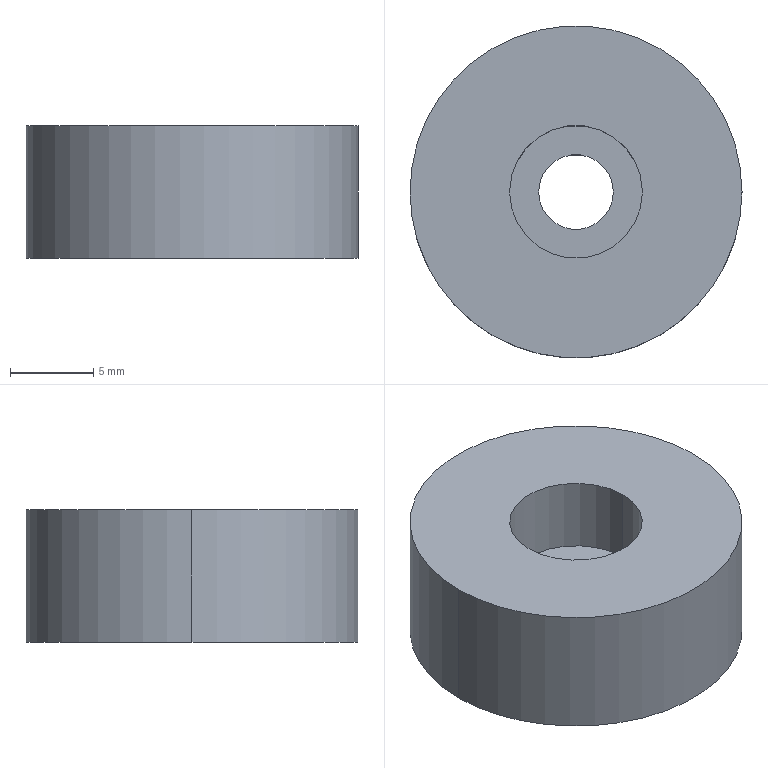Part | STEP file | X77-04005 | 1 solid | 12 faces | box 20 x 20 x 8 mm | volume 2090 mm3 | cylinder 8 | plane 4 | commonest cylinder face diameters 4.5 x2 8 x2 14 x2 20 x2
STEP:
#1=CARTESIAN_POINT('',(7.,0.,1.));
#2=VERTEX_POINT('',#1);
#3=CARTESIAN_POINT('',(-7.,0.,1.));
#4=VERTEX_POINT('',#3);
#5=CARTESIAN_POINT('',(0.,0.,1.));
#6=DIRECTION('',(0.,0.,-1.));
#7=DIRECTION('',(-1.,0.,0.));
#8=AXIS2_PLACEMENT_3D('',#5,#6,#7);
#9=CIRCLE('',#8,7.);
#10=EDGE_CURVE('',#2,#4,#9,.T.);
#11=ORIENTED_EDGE('',*,*,#10,.F.);
#12=CARTESIAN_POINT('',(7.,0.,0.));
#13=VERTEX_POINT('',#12);
#14=CARTESIAN_POINT('',(7.,0.,1.));
#15=DIRECTION('',(0.,0.,-1.));
#16=VECTOR('',#15,1000.);
#17=LINE('',#14,#16);
#18=EDGE_CURVE('',#2,#13,#17,.T.);
#19=ORIENTED_EDGE('',*,*,#18,.T.);
#20=CARTESIAN_POINT('',(-7.,0.,0.));
#21=VERTEX_POINT('',#20);
#22=CARTESIAN_POINT('',(0.,0.,0.));
#23=DIRECTION('',(0.,0.,-1.));
#24=DIRECTION('',(-1.,0.,0.));
#25=AXIS2_PLACEMENT_3D('',#22,#23,#24);
#26=CIRCLE('',#25,7.);
#27=EDGE_CURVE('',#13,#21,#26,.T.);
#28=ORIENTED_EDGE('',*,*,#27,.T.);
#29=CARTESIAN_POINT('',(-7.,0.,1.));
#30=DIRECTION('',(0.,0.,-1.));
#31=VECTOR('',#30,1000.);
#32=LINE('',#29,#31);
#33=EDGE_CURVE('',#4,#21,#32,.T.);
#34=ORIENTED_EDGE('',*,*,#33,.F.);
#35=EDGE_LOOP('',(#11,#19,#28,#34));
#36=FACE_OUTER_BOUND('',#35,.T.);
#37=CARTESIAN_POINT('',(0.,0.,1.));
#38=DIRECTION('',(0.,0.,-1.));
#39=DIRECTION('',(-1.,0.,0.));
#40=AXIS2_PLACEMENT_3D('',#37,#38,#39);
#41=CYLINDRICAL_SURFACE('',#40,7.);
#42=ADVANCED_FACE('',(#36),#41,.F.);
#43=CARTESIAN_POINT('',(-4.,0.,3.4));
#44=VERTEX_POINT('',#43);
#45=CARTESIAN_POINT('',(4.,0.,3.4));
#46=VERTEX_POINT('',#45);
#47=CARTESIAN_POINT('',(0.,0.,3.4));
#48=DIRECTION('',(0.,0.,1.));
#49=DIRECTION('',(1.,0.,0.));
#50=AXIS2_PLACEMENT_3D('',#47,#48,#49);
#51=CIRCLE('',#50,4.);
#52=EDGE_CURVE('',#44,#46,#51,.T.);
#53=ORIENTED_EDGE('',*,*,#52,.F.);
#54=CARTESIAN_POINT('',(-4.,0.,8.));
#55=VERTEX_POINT('',#54);
#56=CARTESIAN_POINT('',(-4.,0.,8.));
#57=DIRECTION('',(0.,0.,1.));
#58=VECTOR('',#57,1000.);
#59=LINE('',#56,#58);
#60=EDGE_CURVE('',#44,#55,#59,.T.);
#61=ORIENTED_EDGE('',*,*,#60,.T.);
#62=CARTESIAN_POINT('',(4.,0.,8.));
#63=VERTEX_POINT('',#62);
#64=CARTESIAN_POINT('',(0.,0.,8.));
#65=DIRECTION('',(0.,0.,1.));
#66=DIRECTION('',(1.,0.,0.));
#67=AXIS2_PLACEMENT_3D('',#64,#65,#66);
#68=CIRCLE('',#67,4.);
#69=EDGE_CURVE('',#55,#63,#68,.T.);
#70=ORIENTED_EDGE('',*,*,#69,.T.);
#71=CARTESIAN_POINT('',(4.,0.,8.));
#72=DIRECTION('',(0.,0.,1.));
#73=VECTOR('',#72,1000.);
#74=LINE('',#71,#73);
#75=EDGE_CURVE('',#46,#63,#74,.T.);
#76=ORIENTED_EDGE('',*,*,#75,.F.);
#77=EDGE_LOOP('',(#53,#61,#70,#76));
#78=FACE_OUTER_BOUND('',#77,.T.);
#79=CARTESIAN_POINT('',(0.,0.,8.));
#80=DIRECTION('',(0.,0.,1.));
#81=DIRECTION('',(1.,0.,0.));
#82=AXIS2_PLACEMENT_3D('',#79,#80,#81);
#83=CYLINDRICAL_SURFACE('',#82,4.);
#84=ADVANCED_FACE('',(#78),#83,.F.);
#85=CARTESIAN_POINT('',(10.,0.,8.));
#86=VERTEX_POINT('',#85);
#87=CARTESIAN_POINT('',(-10.,0.,8.));
#88=VERTEX_POINT('',#87);
#89=CARTESIAN_POINT('',(0.,0.,8.));
#90=DIRECTION('',(0.,0.,1.));
#91=DIRECTION('',(1.,0.,0.));
#92=AXIS2_PLACEMENT_3D('',#89,#90,#91);
#93=CIRCLE('',#92,10.);
#94=EDGE_CURVE('',#86,#88,#93,.T.);
#95=ORIENTED_EDGE('',*,*,#94,.F.);
#96=CARTESIAN_POINT('',(10.,0.,0.));
#97=VERTEX_POINT('',#96);
#98=CARTESIAN_POINT('',(10.,0.,8.));
#99=DIRECTION('',(0.,0.,-1.));
#100=VECTOR('',#99,1000.);
#101=LINE('',#98,#100);
#102=EDGE_CURVE('',#86,#97,#101,.T.);
#103=ORIENTED_EDGE('',*,*,#102,.T.);
#104=CARTESIAN_POINT('',(-10.,0.,0.));
#105=VERTEX_POINT('',#104);
#106=CARTESIAN_POINT('',(0.,0.,0.));
#107=DIRECTION('',(0.,0.,1.));
#108=DIRECTION('',(1.,0.,0.));
#109=AXIS2_PLACEMENT_3D('',#106,#107,#108);
#110=CIRCLE('',#109,10.);
#111=EDGE_CURVE('',#97,#105,#110,.T.);
#112=ORIENTED_EDGE('',*,*,#111,.T.);
#113=CARTESIAN_POINT('',(-10.,0.,8.));
#114=DIRECTION('',(0.,0.,-1.));
#115=VECTOR('',#114,1000.);
#116=LINE('',#113,#115);
#117=EDGE_CURVE('',#88,#105,#116,.T.);
#118=ORIENTED_EDGE('',*,*,#117,.F.);
#119=EDGE_LOOP('',(#95,#103,#112,#118));
#120=FACE_OUTER_BOUND('',#119,.T.);
#121=CARTESIAN_POINT('',(0.,0.,8.));
#122=DIRECTION('',(0.,0.,-1.));
#123=DIRECTION('',(-1.,0.,0.));
#124=AXIS2_PLACEMENT_3D('',#121,#122,#123);
#125=CYLINDRICAL_SURFACE('',#124,10.);
#126=ADVANCED_FACE('',(#120),#125,.T.);
#127=CARTESIAN_POINT('',(-2.25,0.,1.));
#128=VERTEX_POINT('',#127);
#129=CARTESIAN_POINT('',(2.25,0.,1.));
#130=VERTEX_POINT('',#129);
#131=CARTESIAN_POINT('',(0.,0.,1.));
#132=DIRECTION('',(0.,0.,1.));
#133=DIRECTION('',(-1.,0.,0.));
#134=AXIS2_PLACEMENT_3D('',#131,#132,#133);
#135=CIRCLE('',#134,2.25);
#136=EDGE_CURVE('',#128,#130,#135,.T.);
#137=ORIENTED_EDGE('',*,*,#136,.F.);
#138=CARTESIAN_POINT('',(-2.25,0.,3.4));
#139=VERTEX_POINT('',#138);
#140=CARTESIAN_POINT('',(-2.25,0.,8.));
#141=DIRECTION('',(0.,0.,1.));
#142=VECTOR('',#141,1000.);
#143=LINE('',#140,#142);
#144=EDGE_CURVE('',#128,#139,#143,.T.);
#145=ORIENTED_EDGE('',*,*,#144,.T.);
#146=CARTESIAN_POINT('',(2.25,0.,3.4));
#147=VERTEX_POINT('',#146);
#148=CARTESIAN_POINT('',(0.,0.,3.4));
#149=DIRECTION('',(0.,0.,1.));
#150=DIRECTION('',(1.,0.,0.));
#151=AXIS2_PLACEMENT_3D('',#148,#149,#150);
#152=CIRCLE('',#151,2.25);
#153=EDGE_CURVE('',#139,#147,#152,.T.);
#154=ORIENTED_EDGE('',*,*,#153,.T.);
#155=CARTESIAN_POINT('',(2.25,0.,8.));
#156=DIRECTION('',(0.,0.,1.));
#157=VECTOR('',#156,1000.);
#158=LINE('',#155,#157);
#159=EDGE_CURVE('',#130,#147,#158,.T.);
#160=ORIENTED_EDGE('',*,*,#159,.F.);
#161=EDGE_LOOP('',(#137,#145,#154,#160));
#162=FACE_OUTER_BOUND('',#161,.T.);
#163=CARTESIAN_POINT('',(0.,0.,8.));
#164=DIRECTION('',(0.,0.,1.));
#165=DIRECTION('',(1.,0.,0.));
#166=AXIS2_PLACEMENT_3D('',#163,#164,#165);
#167=CYLINDRICAL_SURFACE('',#166,2.25);
#168=ADVANCED_FACE('',(#162),#167,.F.);
#169=ORIENTED_EDGE('',*,*,#144,.F.);
#170=CARTESIAN_POINT('',(0.,0.,1.));
#171=DIRECTION('',(0.,0.,1.));
#172=DIRECTION('',(-1.,0.,0.));
#173=AXIS2_PLACEMENT_3D('',#170,#171,#172);
#174=CIRCLE('',#173,2.25);
#175=EDGE_CURVE('',#130,#128,#174,.T.);
#176=ORIENTED_EDGE('',*,*,#175,.F.);
#177=ORIENTED_EDGE('',*,*,#159,.T.);
#178=CARTESIAN_POINT('',(0.,0.,3.4));
#179=DIRECTION('',(0.,0.,1.));
#180=DIRECTION('',(1.,0.,0.));
#181=AXIS2_PLACEMENT_3D('',#178,#179,#180);
#182=CIRCLE('',#181,2.25);
#183=EDGE_CURVE('',#147,#139,#182,.T.);
#184=ORIENTED_EDGE('',*,*,#183,.T.);
#185=EDGE_LOOP('',(#169,#176,#177,#184));
#186=FACE_OUTER_BOUND('',#185,.T.);
#187=CARTESIAN_POINT('',(0.,0.,8.));
#188=DIRECTION('',(0.,0.,1.));
#189=DIRECTION('',(1.,0.,0.));
#190=AXIS2_PLACEMENT_3D('',#187,#188,#189);
#191=CYLINDRICAL_SURFACE('',#190,2.25);
#192=ADVANCED_FACE('',(#186),#191,.F.);
#193=ORIENTED_EDGE('',*,*,#102,.F.);
#194=CARTESIAN_POINT('',(0.,0.,8.));
#195=DIRECTION('',(0.,0.,1.));
#196=DIRECTION('',(1.,0.,0.));
#197=AXIS2_PLACEMENT_3D('',#194,#195,#196);
#198=CIRCLE('',#197,10.);
#199=EDGE_CURVE('',#88,#86,#198,.T.);
#200=ORIENTED_EDGE('',*,*,#199,.F.);
#201=ORIENTED_EDGE('',*,*,#117,.T.);
#202=CARTESIAN_POINT('',(0.,0.,0.));
#203=DIRECTION('',(0.,0.,1.));
#204=DIRECTION('',(1.,0.,0.));
#205=AXIS2_PLACEMENT_3D('',#202,#203,#204);
#206=CIRCLE('',#205,10.);
#207=EDGE_CURVE('',#105,#97,#206,.T.);
#208=ORIENTED_EDGE('',*,*,#207,.T.);
#209=EDGE_LOOP('',(#193,#200,#201,#208));
#210=FACE_OUTER_BOUND('',#209,.T.);
#211=CARTESIAN_POINT('',(0.,0.,8.));
#212=DIRECTION('',(0.,0.,-1.));
#213=DIRECTION('',(-1.,0.,0.));
#214=AXIS2_PLACEMENT_3D('',#211,#212,#213);
#215=CYLINDRICAL_SURFACE('',#214,10.);
#216=ADVANCED_FACE('',(#210),#215,.T.);
#217=CARTESIAN_POINT('',(0.,0.,8.));
#218=DIRECTION('',(0.,0.,1.));
#219=DIRECTION('',(1.,0.,0.));
#220=AXIS2_PLACEMENT_3D('',#217,#218,#219);
#221=CIRCLE('',#220,4.);
#222=EDGE_CURVE('',#63,#55,#221,.T.);
#223=ORIENTED_EDGE('',*,*,#222,.F.);
#224=ORIENTED_EDGE('',*,*,#69,.F.);
#225=EDGE_LOOP('',(#223,#224));
#226=FACE_BOUND('',#225,.T.);
#227=ORIENTED_EDGE('',*,*,#199,.T.);
#228=ORIENTED_EDGE('',*,*,#94,.T.);
#229=EDGE_LOOP('',(#227,#228));
#230=FACE_OUTER_BOUND('',#229,.T.);
#231=CARTESIAN_POINT('',(0.,0.,8.));
#232=DIRECTION('',(0.,0.,1.));
#233=DIRECTION('',(1.,0.,0.));
#234=AXIS2_PLACEMENT_3D('',#231,#232,#233);
#235=PLANE('',#234);
#236=ADVANCED_FACE('',(#226,#230),#235,.T.);
#237=CARTESIAN_POINT('',(0.,0.,0.));
#238=DIRECTION('',(0.,0.,-1.));
#239=DIRECTION('',(-1.,0.,0.));
#240=AXIS2_PLACEMENT_3D('',#237,#238,#239);
#241=CIRCLE('',#240,7.);
#242=EDGE_CURVE('',#21,#13,#241,.T.);
#243=ORIENTED_EDGE('',*,*,#242,.F.);
#244=ORIENTED_EDGE('',*,*,#27,.F.);
#245=EDGE_LOOP('',(#243,#244));
#246=FACE_BOUND('',#245,.T.);
#247=ORIENTED_EDGE('',*,*,#207,.F.);
#248=ORIENTED_EDGE('',*,*,#111,.F.);
#249=EDGE_LOOP('',(#247,#248));
#250=FACE_OUTER_BOUND('',#249,.T.);
#251=CARTESIAN_POINT('',(0.,0.,0.));
#252=DIRECTION('',(0.,0.,1.));
#253=DIRECTION('',(1.,0.,0.));
#254=AXIS2_PLACEMENT_3D('',#251,#252,#253);
#255=PLANE('',#254);
#256=ADVANCED_FACE('',(#246,#250),#255,.F.);
#257=ORIENTED_EDGE('',*,*,#183,.F.);
#258=ORIENTED_EDGE('',*,*,#153,.F.);
#259=EDGE_LOOP('',(#257,#258));
#260=FACE_BOUND('',#259,.T.);
#261=CARTESIAN_POINT('',(0.,0.,3.4));
#262=DIRECTION('',(0.,0.,1.));
#263=DIRECTION('',(1.,0.,0.));
#264=AXIS2_PLACEMENT_3D('',#261,#262,#263);
#265=CIRCLE('',#264,4.);
#266=EDGE_CURVE('',#46,#44,#265,.T.);
#267=ORIENTED_EDGE('',*,*,#266,.T.);
#268=ORIENTED_EDGE('',*,*,#52,.T.);
#269=EDGE_LOOP('',(#267,#268));
#270=FACE_OUTER_BOUND('',#269,.T.);
#271=CARTESIAN_POINT('',(2.25,0.,3.4));
#272=DIRECTION('',(0.,0.,-1.));
#273=DIRECTION('',(-1.,0.,0.));
#274=AXIS2_PLACEMENT_3D('',#271,#272,#273);
#275=PLANE('',#274);
#276=ADVANCED_FACE('',(#260,#270),#275,.F.);
#277=ORIENTED_EDGE('',*,*,#60,.F.);
#278=ORIENTED_EDGE('',*,*,#266,.F.);
#279=ORIENTED_EDGE('',*,*,#75,.T.);
#280=ORIENTED_EDGE('',*,*,#222,.T.);
#281=EDGE_LOOP('',(#277,#278,#279,#280));
#282=FACE_OUTER_BOUND('',#281,.T.);
#283=CARTESIAN_POINT('',(0.,0.,8.));
#284=DIRECTION('',(0.,0.,1.));
#285=DIRECTION('',(1.,0.,0.));
#286=AXIS2_PLACEMENT_3D('',#283,#284,#285);
#287=CYLINDRICAL_SURFACE('',#286,4.);
#288=ADVANCED_FACE('',(#282),#287,.F.);
#289=CARTESIAN_POINT('',(0.,0.,1.));
#290=DIRECTION('',(0.,0.,-1.));
#291=DIRECTION('',(-1.,0.,0.));
#292=AXIS2_PLACEMENT_3D('',#289,#290,#291);
#293=CIRCLE('',#292,7.);
#294=EDGE_CURVE('',#4,#2,#293,.T.);
#295=ORIENTED_EDGE('',*,*,#294,.T.);
#296=ORIENTED_EDGE('',*,*,#10,.T.);
#297=EDGE_LOOP('',(#295,#296));
#298=FACE_OUTER_BOUND('',#297,.T.);
#299=ORIENTED_EDGE('',*,*,#175,.T.);
#300=ORIENTED_EDGE('',*,*,#136,.T.);
#301=EDGE_LOOP('',(#299,#300));
#302=FACE_BOUND('',#301,.T.);
#303=CARTESIAN_POINT('',(0.,0.,1.));
#304=DIRECTION('',(0.,0.,-1.));
#305=DIRECTION('',(-1.,0.,0.));
#306=AXIS2_PLACEMENT_3D('',#303,#304,#305);
#307=PLANE('',#306);
#308=ADVANCED_FACE('',(#298,#302),#307,.T.);
#309=ORIENTED_EDGE('',*,*,#18,.F.);
#310=ORIENTED_EDGE('',*,*,#294,.F.);
#311=ORIENTED_EDGE('',*,*,#33,.T.);
#312=ORIENTED_EDGE('',*,*,#242,.T.);
#313=EDGE_LOOP('',(#309,#310,#311,#312));
#314=FACE_OUTER_BOUND('',#313,.T.);
#315=CARTESIAN_POINT('',(0.,0.,1.));
#316=DIRECTION('',(0.,0.,-1.));
#317=DIRECTION('',(-1.,0.,0.));
#318=AXIS2_PLACEMENT_3D('',#315,#316,#317);
#319=CYLINDRICAL_SURFACE('',#318,7.);
#320=ADVANCED_FACE('',(#314),#319,.F.);
#321=CLOSED_SHELL('',(#42,#84,#126,#168,#192,#216,#236,#256,#276,#288,#308,#320));
#322=MANIFOLD_SOLID_BREP('',#321);
#323=CARTESIAN_POINT('',(0.,0.,0.));
#324=DIRECTION('',(0.,0.,1.));
#325=DIRECTION('',(1.,0.,0.));
#326=AXIS2_PLACEMENT_3D('',#323,#324,#325);
#327=(LENGTH_UNIT()NAMED_UNIT(*)SI_UNIT(.MILLI.,.METRE.));
#328=UNCERTAINTY_MEASURE_WITH_UNIT(LENGTH_MEASURE(0.00001),#327,'','');
#329=(NAMED_UNIT(*)PLANE_ANGLE_UNIT()SI_UNIT($,.RADIAN.));
#330=(NAMED_UNIT(*)SI_UNIT($,.STERADIAN.)SOLID_ANGLE_UNIT());
#331=(GEOMETRIC_REPRESENTATION_CONTEXT(3)GLOBAL_UNCERTAINTY_ASSIGNED_CONTEXT((#328))GLOBAL_UNIT_ASSIGNED_CONTEXT((#327,#329,#330))REPRESENTATION_CONTEXT('',''));
#332=ADVANCED_BREP_SHAPE_REPRESENTATION('',(#322,#326),#331);